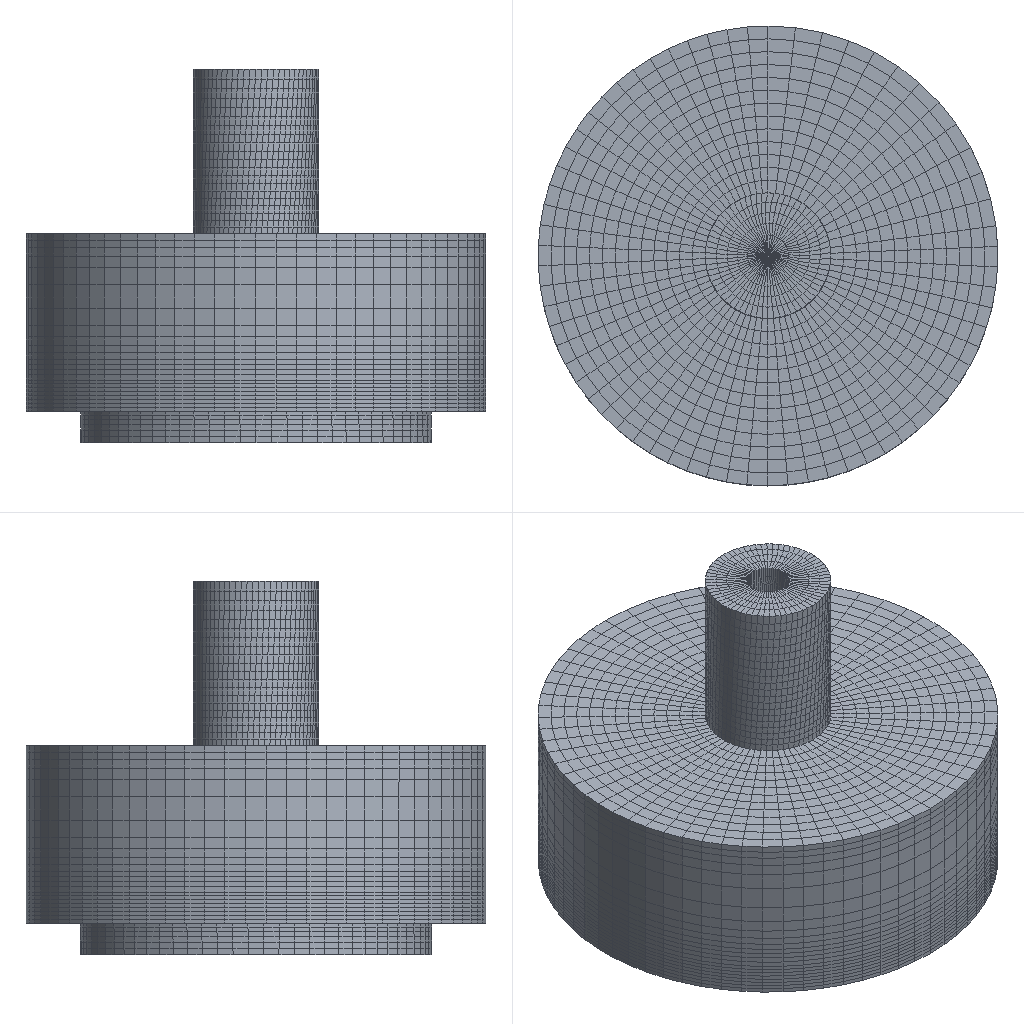Simulation study | ansys fluent
Set-up summary, first 114 of 241 lines:
category,name,step,type,value,unit,region
solver,ansys_fluent,,Fluent 26.1.0
units,SI m-kg-s (Fluent internal),,stated,boundary values in the units shown in brackets; results in listed units
analysis,deck-1.cas,,cfd steady,"dimension=3D; solver=3d, dp, pbns, spe, lam (3d, double precision, pressure-based,  species, laminar); source_case=2.cas"
model,Space,deck-1.cas,,3D
model,Time,deck-1.cas,,Steady
model,Viscous,deck-1.cas,,Laminar
model,Heat Transfer,deck-1.cas,,Enabled
model,Species,deck-1.cas,,Reacting (4 species)
model,Multiphase,deck-1.cas,,Disabled
analysis,deck-2.cas,,cfd steady,"dimension=3D; solver=3d, dp, pbns, spe, lam (3d, double precision, pressure-based,  species, laminar); source_case=.cas.h5"
model,Space,deck-2.cas,,3D
model,Time,deck-2.cas,,Steady
model,Viscous,deck-2.cas,,Laminar
model,Heat Transfer,deck-2.cas,,Enabled
model,Species,deck-2.cas,,Reacting (4 species)
model,Multiphase,deck-2.cas,,Disabled
mesh,deck-1.cas,,nodes,43245
mesh,deck-1.cas,,elements,38478
mesh,deck-1.cas,,faces,120186
mesh,deck-1.cas,,note,elements = cells; counts from the case file zone headers
mesh,deck-2.cas,,nodes,43245
mesh,deck-2.cas,,elements,38478
mesh,deck-2.cas,,faces,120186
mesh,deck-2.cas,,note,elements = cells; counts from the case file zone headers
cell_zone,fluid,deck-1.cas,fluid,material=gaas_deposition,,zone 2
cell_zone,fluid,deck-2.cas,fluid,material=gaas_deposition,,zone 2
material,water-vapor (fluid),,Density,0.5542,kg/m^3
material,water-vapor (fluid),,Cp (Specific Heat),piecewise-polynomial: (300-1000: 1563.077 1.604 -0.002933 3.2161009e-06 -1.1568268e-09) (1000-5000: 1233.234 1.411 -0.0004029 5.5427718e-08 -2.949824e-12),J/(kg K)
material,water-vapor (fluid),,Thermal Conductivity,0.0261,W/(m K)
material,water-vapor (fluid),,Viscosity,1.34e-05,kg/(m s)
material,water-vapor (fluid),,Molecular Weight,18.015,kg/kmol
material,water-vapor (fluid),,Standard State Enthalpy,-2.418379e+08,J/kgmol
material,water-vapor (fluid),,Standard State Entropy,188696.44,J/(kgmol K)
material,water-vapor (fluid),,Reference Temperature,298.15,K
material,oxygen (fluid),,Density,1.3,kg/m^3
material,oxygen (fluid),,Cp (Specific Heat),piecewise-polynomial: (300-1000: 834.826 0.293 -0.0001496 3.4138849e-07 -2.2783585e-10) (1000-5000: 960.752 0.1594 -3.2708852e-05 4.6127648e-09 -2.9528324e-13),J/(kg K)
material,oxygen (fluid),,Thermal Conductivity,0.0246,W/(m K)
material,oxygen (fluid),,Viscosity,1.919e-05,kg/(m s)
material,oxygen (fluid),,Molecular Weight,31.999,kg/kmol
material,oxygen (fluid),,Standard State Enthalpy,0,J/kgmol
material,oxygen (fluid),,Standard State Entropy,205026.86,J/(kgmol K)
material,oxygen (fluid),,Reference Temperature,298.15,K
material,nitrogen (fluid),,Density,1.138,kg/m^3
material,nitrogen (fluid),,Cp (Specific Heat),piecewise-polynomial: (300-1000: 979.043 0.418 -0.001176 1.6743943e-06 -7.2562971e-10) (1000-5000: 868.623 0.4416 -0.0001687 2.9967875e-08 -2.0043858e-12),J/(kg K)
material,nitrogen (fluid),,Thermal Conductivity,0.0242,W/(m K)
material,nitrogen (fluid),,Viscosity,1.663e-05,kg/(m s)
material,nitrogen (fluid),,Molecular Weight,28.013,kg/kmol
material,nitrogen (fluid),,Standard State Enthalpy,0,J/kgmol
material,nitrogen (fluid),,Standard State Entropy,191494.78,J/(kgmol K)
material,nitrogen (fluid),,Reference Temperature,298.15,K
material,(as_s . gaas_deposition) (fluid),,Cp (Specific Heat),520.64,J/(kg K)
material,(as_s . gaas_deposition) (fluid),,Thermal Conductivity,0.0158,W/(m K)
material,(as_s . gaas_deposition) (fluid),,Viscosity,2.125,kg/(m s)
material,(as_s . gaas_deposition) (fluid),,Molecular Weight,74.92,kg/kmol
material,(as_s . gaas_deposition) (fluid),,Standard State Enthalpy,-3117.71,J/kgmol
material,(as_s . gaas_deposition) (fluid),,Standard State Entropy,154719.3,J/(kgmol K)
material,(as_s . gaas_deposition) (fluid),,Reference Temperature,298.15,K
material,(as_s . gaas_deposition) (fluid),,L-J Characteristic Length,3.711,Angstrom
material,(as_s . gaas_deposition) (fluid),,L-J Energy Parameter,78.6,K
material,(ga_s . gaas_deposition) (fluid),,Cp (Specific Heat),520.64,J/(kg K)
material,(ga_s . gaas_deposition) (fluid),,Thermal Conductivity,0.0158,W/(m K)
material,(ga_s . gaas_deposition) (fluid),,Viscosity,2.125,kg/(m s)
material,(ga_s . gaas_deposition) (fluid),,Molecular Weight,69.72,kg/kmol
material,(ga_s . gaas_deposition) (fluid),,Standard State Enthalpy,-3117.71,J/kgmol
material,(ga_s . gaas_deposition) (fluid),,Standard State Entropy,154719.3,J/(kgmol K)
material,(ga_s . gaas_deposition) (fluid),,Reference Temperature,298.15,K
material,(ga_s . gaas_deposition) (fluid),,L-J Characteristic Length,3.711,Angstrom
material,(ga_s . gaas_deposition) (fluid),,L-J Energy Parameter,78.6,K
material,(as . gaas_deposition) (fluid),,Cp (Specific Heat),1006.43,J/(kg K)
material,(as . gaas_deposition) (fluid),,Thermal Conductivity,kinetic-theory: #f,W/(m K)
material,(as . gaas_deposition) (fluid),,Viscosity,kinetic-theory: #f,kg/(m s)
material,(as . gaas_deposition) (fluid),,Molecular Weight,74.92,kg/kmol
material,(as . gaas_deposition) (fluid),,Standard State Enthalpy,0,J/kgmol
material,(as . gaas_deposition) (fluid),,Standard State Entropy,0,J/(kgmol K)
material,(as . gaas_deposition) (fluid),,Reference Temperature,298.15,K
material,(as . gaas_deposition) (fluid),,L-J Characteristic Length,0,Angstrom
material,(as . gaas_deposition) (fluid),,L-J Energy Parameter,0,K
material,(ga . gaas_deposition) (fluid),,Cp (Specific Heat),1006.43,J/(kg K)
material,(ga . gaas_deposition) (fluid),,Thermal Conductivity,kinetic-theory: #f,W/(m K)
material,(ga . gaas_deposition) (fluid),,Viscosity,kinetic-theory: #f,kg/(m s)
material,(ga . gaas_deposition) (fluid),,Molecular Weight,69.72,kg/kmol
material,(ga . gaas_deposition) (fluid),,Standard State Enthalpy,0,J/kgmol
material,(ga . gaas_deposition) (fluid),,Standard State Entropy,0,J/(kgmol K)
material,(ga . gaas_deposition) (fluid),,Reference Temperature,298.15,K
material,(ga . gaas_deposition) (fluid),,L-J Characteristic Length,0,Angstrom
material,(ga . gaas_deposition) (fluid),,L-J Energy Parameter,0,K
material,(hydrogen . gaas_deposition) (fluid),,Cp (Specific Heat),kinetic-theory: #f,J/(kg K)
material,(hydrogen . gaas_deposition) (fluid),,Thermal Conductivity,kinetic-theory: #f,W/(m K)
material,(hydrogen . gaas_deposition) (fluid),,Viscosity,kinetic-theory: #f,kg/(m s)
material,(hydrogen . gaas_deposition) (fluid),,Molecular Weight,2.02,kg/kmol
material,(hydrogen . gaas_deposition) (fluid),,Standard State Enthalpy,0,J/kgmol
material,(hydrogen . gaas_deposition) (fluid),,Standard State Entropy,130579.1,J/(kgmol K)
material,(hydrogen . gaas_deposition) (fluid),,Reference Temperature,298.15,K
material,(hydrogen . gaas_deposition) (fluid),,L-J Characteristic Length,2.827,Angstrom
material,(hydrogen . gaas_deposition) (fluid),,L-J Energy Parameter,59.7,K
material,(hydrogen . gaas_deposition) (fluid),,Degrees of Freedom,5
material,(ch3g . gaas_deposition) (fluid),,Cp (Specific Heat),kinetic-theory: #f,J/(kg K)
material,(ch3g . gaas_deposition) (fluid),,Thermal Conductivity,kinetic-theory: #f,W/(m K)
material,(ch3g . gaas_deposition) (fluid),,Viscosity,kinetic-theory: #f,kg/(m s)
material,(ch3g . gaas_deposition) (fluid),,Molecular Weight,15,kg/kmol
material,(ch3g . gaas_deposition) (fluid),,Standard State Enthalpy,2.044,J/kgmol
material,(ch3g . gaas_deposition) (fluid),,Standard State Entropy,257367.59,J/(kgmol K)
material,(ch3g . gaas_deposition) (fluid),,Reference Temperature,298.15,K
material,(ch3g . gaas_deposition) (fluid),,L-J Characteristic Length,3.758,Angstrom
material,(ch3g . gaas_deposition) (fluid),,L-J Energy Parameter,148.6,K
material,(ch3g . gaas_deposition) (fluid),,Degrees of Freedom,0
material,(tmg . gaas_deposition) (fluid),,Cp (Specific Heat),kinetic-theory: #f,J/(kg K)
material,(tmg . gaas_deposition) (fluid),,Thermal Conductivity,kinetic-theory: #f,W/(m K)
material,(tmg . gaas_deposition) (fluid),,Viscosity,kinetic-theory: #f,kg/(m s)
material,(tmg . gaas_deposition) (fluid),,Molecular Weight,114.83,kg/kmol
material,(tmg . gaas_deposition) (fluid),,Standard State Enthalpy,0,J/kgmol
material,(tmg . gaas_deposition) (fluid),,Standard State Entropy,130579.1,J/(kgmol K)
material,(tmg . gaas_deposition) (fluid),,Reference Temperature,298.15,K
Results summary, first 52 of 68 lines:
result,mass flow rate outlet,deck-1.cas,,-4.62764e-05,kg/s
result,mass flow rate velocity-inlet,deck-1.cas,,5.59628e-05,kg/s
result,mass flow rate wall-1,deck-1.cas,,-0,kg/s
result,mass flow rate wall-2,deck-1.cas,,-0,kg/s
result,mass flow rate wall-4,deck-1.cas,,-9.68641e-06,kg/s
result,mass flow rate wall-5,deck-1.cas,,-0,kg/s
result,mass flow rate wall-6,deck-1.cas,,-0,kg/s
result,mass flow rate Net,deck-1.cas,,-2.48484e-11,kg/s
result,heat transfer rate outlet,deck-1.cas,,-66.8,W
result,heat transfer rate velocity-inlet,deck-1.cas,,-211.606,W
result,heat transfer rate wall-1,deck-1.cas,,-170.461,W
result,heat transfer rate wall-2,deck-1.cas,,-1372.08,W
result,heat transfer rate wall-4,deck-1.cas,,1958.27,W
result,heat transfer rate wall-5,deck-1.cas,,144.685,W
result,heat transfer rate wall-6,deck-1.cas,,-282.004,W
result,heat transfer rate Net,deck-1.cas,,6.33126e-05,W
result,wall force total wall-1,deck-1.cas,,"(9.13235e-06, 6.1479e-06, -0.006118)",N
result,wall force pressure wall-1,deck-1.cas,,"(5.91638e-06, 2.57554e-06, -0.006021)",N
result,wall force viscous wall-1,deck-1.cas,,"(3.21596e-06, 3.57236e-06, -9.7845e-05)",N
result,wall force total wall-2,deck-1.cas,,"(2.91366e-05, -5.0228e-05, 0.0005938)",N
result,wall force pressure wall-2,deck-1.cas,,"(2.20263e-05, -5.04887e-05, 2.85665e-09)",N
result,wall force viscous wall-2,deck-1.cas,,"(7.11023e-06, 2.60667e-07, 0.0005938)",N
result,wall force total wall-4,deck-1.cas,,"(-3.38849e-05, 3.7089e-05, -0.002756)",N
result,wall force pressure wall-4,deck-1.cas,,"(-5.91074e-06, -1.03592e-06, -0.00274)",N
result,wall force viscous wall-4,deck-1.cas,,"(-2.79741e-05, 3.81249e-05, -1.62661e-05)",N
result,wall force total wall-5,deck-1.cas,,"(-9.38012e-06, 2.9375e-06, -2.4431e-05)",N
result,wall force pressure wall-5,deck-1.cas,,"(-7.61239e-06, 2.36138e-06, 8.06256e-10)",N
result,wall force viscous wall-5,deck-1.cas,,"(-1.76773e-06, 5.76126e-07, -2.44318e-05)",N
result,wall force total wall-6,deck-1.cas,,"(4.9778e-06, 3.63145e-06, 0.008386)",N
result,wall force pressure wall-6,deck-1.cas,,"(1.93923e-11, -7.12933e-12, 0.008336)",N
result,wall force viscous wall-6,deck-1.cas,,"(4.97778e-06, 3.63146e-06, 4.99812e-05)",N
result,wall force total Net,deck-1.cas,,"(-1.82458e-08, -4.22177e-07, 8.07071e-05)",N
result,wall force pressure Net,deck-1.cas,,"(1.44196e-05, -4.65877e-05, -0.0004245)",N
result,wall force viscous Net,deck-1.cas,,"(-1.44379e-05, 4.61655e-05, 0.0005052)",N
result,mass flow rate outlet,deck-2.cas,,-4.62764e-05,kg/s
result,mass flow rate velocity-inlet,deck-2.cas,,5.59628e-05,kg/s
result,mass flow rate wall-1,deck-2.cas,,-0,kg/s
result,mass flow rate wall-2,deck-2.cas,,-0,kg/s
result,mass flow rate wall-4,deck-2.cas,,-9.68641e-06,kg/s
result,mass flow rate wall-5,deck-2.cas,,-0,kg/s
result,mass flow rate wall-6,deck-2.cas,,-0,kg/s
result,mass flow rate Net,deck-2.cas,,-2.48484e-11,kg/s
result,heat transfer rate outlet,deck-2.cas,,-66.8,W
result,heat transfer rate velocity-inlet,deck-2.cas,,-211.606,W
result,heat transfer rate wall-1,deck-2.cas,,-170.461,W
result,heat transfer rate wall-2,deck-2.cas,,-1372.08,W
result,heat transfer rate wall-4,deck-2.cas,,1958.27,W
result,heat transfer rate wall-5,deck-2.cas,,144.685,W
result,heat transfer rate wall-6,deck-2.cas,,-282.004,W
result,heat transfer rate Net,deck-2.cas,,6.33126e-05,W
result,wall force total wall-1,deck-2.cas,,"(9.13235e-06, 6.1479e-06, -0.006118)",N
result,wall force pressure wall-1,deck-2.cas,,"(5.91638e-06, 2.57554e-06, -0.006021)",N